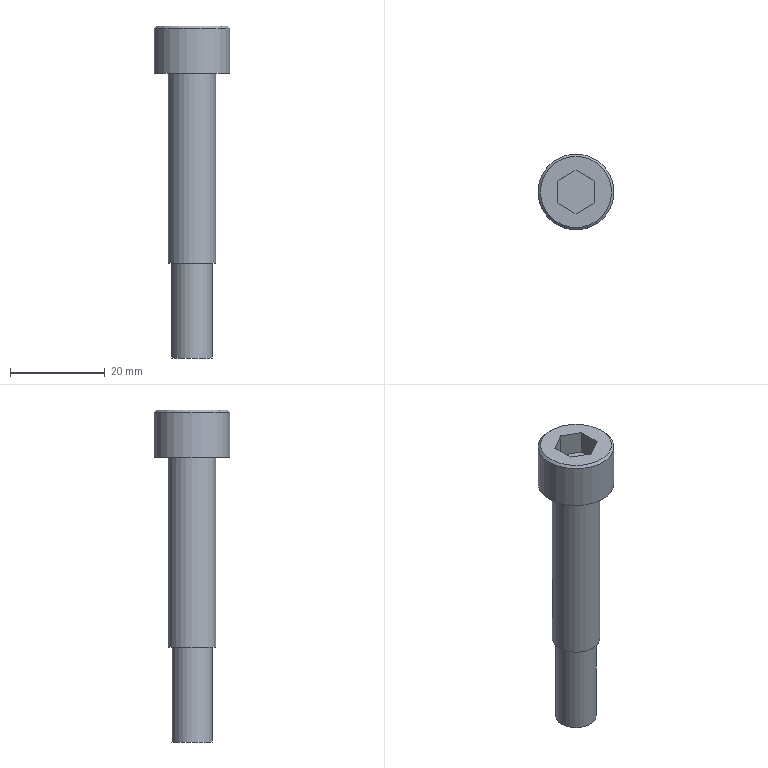Part | STEP file | M6-40_id1114_x_t | 1 solid | 15 faces | box 16 x 16 x 70 mm | volume 6004 mm3 | plane 11 | cylinder 3 | cone 1 | commonest cylinder face diameters 8.5 x1 10 x1 16 x1
STEP:
#1=CARTESIAN_POINT('',(-349.25,-157.5,-47.));
#2=VERTEX_POINT('',#1);
#3=CARTESIAN_POINT('',(-345.,-157.5,-47.));
#4=DIRECTION('',(0.,0.,-1.));
#5=DIRECTION('',(-1.,0.,0.));
#6=AXIS2_PLACEMENT_3D('',#3,#4,#5);
#7=CIRCLE('',#6,4.25);
#8=EDGE_CURVE('',#2,#2,#7,.T.);
#9=ORIENTED_EDGE('',*,*,#8,.F.);
#10=EDGE_LOOP('',(#9));
#11=FACE_BOUND('',#10,.T.);
#12=CARTESIAN_POINT('',(-340.,-157.5,-47.));
#13=VERTEX_POINT('',#12);
#14=CARTESIAN_POINT('',(-345.,-157.5,-47.));
#15=DIRECTION('',(0.,0.,1.));
#16=DIRECTION('',(1.,0.,0.));
#17=AXIS2_PLACEMENT_3D('',#14,#15,#16);
#18=CIRCLE('',#17,5.);
#19=EDGE_CURVE('',#13,#13,#18,.T.);
#20=ORIENTED_EDGE('',*,*,#19,.F.);
#21=EDGE_LOOP('',(#20));
#22=FACE_BOUND('',#21,.T.);
#23=CARTESIAN_POINT('',(-345.,-157.5,-47.));
#24=DIRECTION('',(0.,0.,-1.));
#25=DIRECTION('',(-1.,0.,0.));
#26=AXIS2_PLACEMENT_3D('',#23,#24,#25);
#27=PLANE('',#26);
#28=ADVANCED_FACE('',(#11,#22),#27,.T.);
#29=CARTESIAN_POINT('',(-350.,-157.5,-7.));
#30=VERTEX_POINT('',#29);
#31=CARTESIAN_POINT('',(-345.,-157.5,-7.));
#32=DIRECTION('',(0.,0.,1.));
#33=DIRECTION('',(-1.,0.,0.));
#34=AXIS2_PLACEMENT_3D('',#31,#32,#33);
#35=CIRCLE('',#34,5.);
#36=EDGE_CURVE('',#30,#30,#35,.T.);
#37=ORIENTED_EDGE('',*,*,#36,.F.);
#38=EDGE_LOOP('',(#37));
#39=FACE_BOUND('',#38,.T.);
#40=ORIENTED_EDGE('',*,*,#19,.T.);
#41=EDGE_LOOP('',(#40));
#42=FACE_BOUND('',#41,.T.);
#43=CARTESIAN_POINT('',(-345.,-157.5,-47.));
#44=DIRECTION('',(0.,0.,1.));
#45=DIRECTION('',(1.,0.,0.));
#46=AXIS2_PLACEMENT_3D('',#43,#44,#45);
#47=CYLINDRICAL_SURFACE('',#46,5.);
#48=ADVANCED_FACE('',(#39,#42),#47,.T.);
#49=CARTESIAN_POINT('',(-337.5,-157.5,3.));
#50=VERTEX_POINT('',#49);
#51=CARTESIAN_POINT('',(-345.,-157.5,3.));
#52=DIRECTION('',(0.,0.,1.));
#53=DIRECTION('',(1.,0.,0.));
#54=AXIS2_PLACEMENT_3D('',#51,#52,#53);
#55=CIRCLE('',#54,7.5);
#56=EDGE_CURVE('',#50,#50,#55,.T.);
#57=ORIENTED_EDGE('',*,*,#56,.T.);
#58=EDGE_LOOP('',(#57));
#59=FACE_BOUND('',#58,.T.);
#60=CARTESIAN_POINT('',(-349.,-155.191,3.));
#61=VERTEX_POINT('',#60);
#62=CARTESIAN_POINT('',(-349.,-159.809,3.));
#63=VERTEX_POINT('',#62);
#64=CARTESIAN_POINT('',(-349.,-155.191,3.));
#65=DIRECTION('',(0.,-1.,0.));
#66=VECTOR('',#65,1.);
#67=LINE('',#64,#66);
#68=EDGE_CURVE('',#61,#63,#67,.T.);
#69=ORIENTED_EDGE('',*,*,#68,.F.);
#70=CARTESIAN_POINT('',(-345.,-152.881,3.));
#71=VERTEX_POINT('',#70);
#72=CARTESIAN_POINT('',(-345.,-152.881,3.));
#73=DIRECTION('',(-0.866,-0.5,0.));
#74=VECTOR('',#73,1.);
#75=LINE('',#72,#74);
#76=EDGE_CURVE('',#71,#61,#75,.T.);
#77=ORIENTED_EDGE('',*,*,#76,.F.);
#78=CARTESIAN_POINT('',(-341.,-155.191,3.));
#79=VERTEX_POINT('',#78);
#80=CARTESIAN_POINT('',(-341.,-155.191,3.));
#81=DIRECTION('',(-0.866,0.5,0.));
#82=VECTOR('',#81,1.);
#83=LINE('',#80,#82);
#84=EDGE_CURVE('',#79,#71,#83,.T.);
#85=ORIENTED_EDGE('',*,*,#84,.F.);
#86=CARTESIAN_POINT('',(-341.,-159.809,3.));
#87=VERTEX_POINT('',#86);
#88=CARTESIAN_POINT('',(-341.,-159.809,3.));
#89=DIRECTION('',(0.,1.,0.));
#90=VECTOR('',#89,1.);
#91=LINE('',#88,#90);
#92=EDGE_CURVE('',#87,#79,#91,.T.);
#93=ORIENTED_EDGE('',*,*,#92,.F.);
#94=CARTESIAN_POINT('',(-345.,-162.119,3.));
#95=VERTEX_POINT('',#94);
#96=CARTESIAN_POINT('',(-345.,-162.119,3.));
#97=DIRECTION('',(0.866,0.5,0.));
#98=VECTOR('',#97,1.);
#99=LINE('',#96,#98);
#100=EDGE_CURVE('',#95,#87,#99,.T.);
#101=ORIENTED_EDGE('',*,*,#100,.F.);
#102=CARTESIAN_POINT('',(-349.,-159.809,3.));
#103=DIRECTION('',(0.866,-0.5,0.));
#104=VECTOR('',#103,1.);
#105=LINE('',#102,#104);
#106=EDGE_CURVE('',#63,#95,#105,.T.);
#107=ORIENTED_EDGE('',*,*,#106,.F.);
#108=EDGE_LOOP('',(#69,#77,#85,#93,#101,#107));
#109=FACE_BOUND('',#108,.T.);
#110=CARTESIAN_POINT('',(-345.,-157.5,3.));
#111=DIRECTION('',(0.,0.,1.));
#112=DIRECTION('',(1.,0.,0.));
#113=AXIS2_PLACEMENT_3D('',#110,#111,#112);
#114=PLANE('',#113);
#115=ADVANCED_FACE('',(#59,#109),#114,.T.);
#116=ORIENTED_EDGE('',*,*,#36,.T.);
#117=EDGE_LOOP('',(#116));
#118=FACE_BOUND('',#117,.T.);
#119=CARTESIAN_POINT('',(-337.,-157.5,-7.));
#120=VERTEX_POINT('',#119);
#121=CARTESIAN_POINT('',(-345.,-157.5,-7.));
#122=DIRECTION('',(0.,0.,1.));
#123=DIRECTION('',(1.,0.,0.));
#124=AXIS2_PLACEMENT_3D('',#121,#122,#123);
#125=CIRCLE('',#124,8.);
#126=EDGE_CURVE('',#120,#120,#125,.T.);
#127=ORIENTED_EDGE('',*,*,#126,.F.);
#128=EDGE_LOOP('',(#127));
#129=FACE_BOUND('',#128,.T.);
#130=CARTESIAN_POINT('',(-345.,-157.5,-7.));
#131=DIRECTION('',(0.,0.,-1.));
#132=DIRECTION('',(-1.,0.,0.));
#133=AXIS2_PLACEMENT_3D('',#130,#131,#132);
#134=PLANE('',#133);
#135=ADVANCED_FACE('',(#118,#129),#134,.T.);
#136=CARTESIAN_POINT('',(-337.,-157.5,2.5));
#137=VERTEX_POINT('',#136);
#138=CARTESIAN_POINT('',(-345.,-157.5,2.5));
#139=DIRECTION('',(0.,0.,-1.));
#140=DIRECTION('',(1.,0.,0.));
#141=AXIS2_PLACEMENT_3D('',#138,#139,#140);
#142=CIRCLE('',#141,8.);
#143=EDGE_CURVE('',#137,#137,#142,.T.);
#144=ORIENTED_EDGE('',*,*,#143,.T.);
#145=EDGE_LOOP('',(#144));
#146=FACE_BOUND('',#145,.T.);
#147=ORIENTED_EDGE('',*,*,#126,.T.);
#148=EDGE_LOOP('',(#147));
#149=FACE_BOUND('',#148,.T.);
#150=CARTESIAN_POINT('',(-345.,-157.5,-7.));
#151=DIRECTION('',(0.,0.,1.));
#152=DIRECTION('',(1.,0.,0.));
#153=AXIS2_PLACEMENT_3D('',#150,#151,#152);
#154=CYLINDRICAL_SURFACE('',#153,8.);
#155=ADVANCED_FACE('',(#146,#149),#154,.T.);
#156=CARTESIAN_POINT('',(-340.75,-157.5,-67.));
#157=VERTEX_POINT('',#156);
#158=CARTESIAN_POINT('',(-345.,-157.5,-67.));
#159=DIRECTION('',(0.,0.,1.));
#160=DIRECTION('',(1.,0.,0.));
#161=AXIS2_PLACEMENT_3D('',#158,#159,#160);
#162=CIRCLE('',#161,4.25);
#163=EDGE_CURVE('',#157,#157,#162,.T.);
#164=ORIENTED_EDGE('',*,*,#163,.F.);
#165=EDGE_LOOP('',(#164));
#166=FACE_OUTER_BOUND('',#165,.T.);
#167=CARTESIAN_POINT('',(-345.,-157.5,-67.));
#168=DIRECTION('',(0.,0.,-1.));
#169=DIRECTION('',(-1.,0.,0.));
#170=AXIS2_PLACEMENT_3D('',#167,#168,#169);
#171=PLANE('',#170);
#172=ADVANCED_FACE('',(#166),#171,.T.);
#173=ORIENTED_EDGE('',*,*,#163,.T.);
#174=EDGE_LOOP('',(#173));
#175=FACE_BOUND('',#174,.T.);
#176=ORIENTED_EDGE('',*,*,#8,.T.);
#177=EDGE_LOOP('',(#176));
#178=FACE_BOUND('',#177,.T.);
#179=CARTESIAN_POINT('',(-345.,-157.5,-47.));
#180=DIRECTION('',(0.,0.,-1.));
#181=DIRECTION('',(1.,0.,0.));
#182=AXIS2_PLACEMENT_3D('',#179,#180,#181);
#183=CYLINDRICAL_SURFACE('',#182,4.25);
#184=ADVANCED_FACE('',(#175,#178),#183,.T.);
#185=ORIENTED_EDGE('',*,*,#68,.T.);
#186=CARTESIAN_POINT('',(-349.,-159.809,-2.));
#187=VERTEX_POINT('',#186);
#188=CARTESIAN_POINT('',(-349.,-159.809,-2.));
#189=DIRECTION('',(0.,0.,-1.));
#190=VECTOR('',#189,1.);
#191=LINE('',#188,#190);
#192=EDGE_CURVE('',#63,#187,#191,.T.);
#193=ORIENTED_EDGE('',*,*,#192,.T.);
#194=CARTESIAN_POINT('',(-349.,-155.191,-2.));
#195=VERTEX_POINT('',#194);
#196=CARTESIAN_POINT('',(-349.,-155.191,-2.));
#197=DIRECTION('',(0.,1.,0.));
#198=VECTOR('',#197,1.);
#199=LINE('',#196,#198);
#200=EDGE_CURVE('',#187,#195,#199,.T.);
#201=ORIENTED_EDGE('',*,*,#200,.T.);
#202=CARTESIAN_POINT('',(-349.,-155.191,-2.));
#203=DIRECTION('',(0.,0.,-1.));
#204=VECTOR('',#203,1.);
#205=LINE('',#202,#204);
#206=EDGE_CURVE('',#61,#195,#205,.T.);
#207=ORIENTED_EDGE('',*,*,#206,.F.);
#208=EDGE_LOOP('',(#185,#193,#201,#207));
#209=FACE_OUTER_BOUND('',#208,.T.);
#210=CARTESIAN_POINT('',(-349.,-155.191,-2.));
#211=DIRECTION('',(-1.,0.,0.));
#212=DIRECTION('',(0.,-1.,0.));
#213=AXIS2_PLACEMENT_3D('',#210,#211,#212);
#214=PLANE('',#213);
#215=ADVANCED_FACE('',(#209),#214,.F.);
#216=ORIENTED_EDGE('',*,*,#106,.T.);
#217=CARTESIAN_POINT('',(-345.,-162.119,-2.));
#218=VERTEX_POINT('',#217);
#219=CARTESIAN_POINT('',(-345.,-162.119,-2.));
#220=DIRECTION('',(0.,0.,-1.));
#221=VECTOR('',#220,1.);
#222=LINE('',#219,#221);
#223=EDGE_CURVE('',#95,#218,#222,.T.);
#224=ORIENTED_EDGE('',*,*,#223,.T.);
#225=CARTESIAN_POINT('',(-349.,-159.809,-2.));
#226=DIRECTION('',(-0.866,0.5,0.));
#227=VECTOR('',#226,1.);
#228=LINE('',#225,#227);
#229=EDGE_CURVE('',#218,#187,#228,.T.);
#230=ORIENTED_EDGE('',*,*,#229,.T.);
#231=ORIENTED_EDGE('',*,*,#192,.F.);
#232=EDGE_LOOP('',(#216,#224,#230,#231));
#233=FACE_OUTER_BOUND('',#232,.T.);
#234=CARTESIAN_POINT('',(-349.,-159.809,-2.));
#235=DIRECTION('',(-0.5,-0.866,0.));
#236=DIRECTION('',(0.866,-0.5,0.));
#237=AXIS2_PLACEMENT_3D('',#234,#235,#236);
#238=PLANE('',#237);
#239=ADVANCED_FACE('',(#233),#238,.F.);
#240=ORIENTED_EDGE('',*,*,#100,.T.);
#241=CARTESIAN_POINT('',(-341.,-159.809,-2.));
#242=VERTEX_POINT('',#241);
#243=CARTESIAN_POINT('',(-341.,-159.809,-2.));
#244=DIRECTION('',(0.,0.,-1.));
#245=VECTOR('',#244,1.);
#246=LINE('',#243,#245);
#247=EDGE_CURVE('',#87,#242,#246,.T.);
#248=ORIENTED_EDGE('',*,*,#247,.T.);
#249=CARTESIAN_POINT('',(-345.,-162.119,-2.));
#250=DIRECTION('',(-0.866,-0.5,0.));
#251=VECTOR('',#250,1.);
#252=LINE('',#249,#251);
#253=EDGE_CURVE('',#242,#218,#252,.T.);
#254=ORIENTED_EDGE('',*,*,#253,.T.);
#255=ORIENTED_EDGE('',*,*,#223,.F.);
#256=EDGE_LOOP('',(#240,#248,#254,#255));
#257=FACE_OUTER_BOUND('',#256,.T.);
#258=CARTESIAN_POINT('',(-345.,-162.119,-2.));
#259=DIRECTION('',(0.5,-0.866,0.));
#260=DIRECTION('',(0.866,0.5,0.));
#261=AXIS2_PLACEMENT_3D('',#258,#259,#260);
#262=PLANE('',#261);
#263=ADVANCED_FACE('',(#257),#262,.F.);
#264=ORIENTED_EDGE('',*,*,#92,.T.);
#265=CARTESIAN_POINT('',(-341.,-155.191,-2.));
#266=VERTEX_POINT('',#265);
#267=CARTESIAN_POINT('',(-341.,-155.191,-2.));
#268=DIRECTION('',(0.,0.,-1.));
#269=VECTOR('',#268,1.);
#270=LINE('',#267,#269);
#271=EDGE_CURVE('',#79,#266,#270,.T.);
#272=ORIENTED_EDGE('',*,*,#271,.T.);
#273=CARTESIAN_POINT('',(-341.,-159.809,-2.));
#274=DIRECTION('',(0.,-1.,0.));
#275=VECTOR('',#274,1.);
#276=LINE('',#273,#275);
#277=EDGE_CURVE('',#266,#242,#276,.T.);
#278=ORIENTED_EDGE('',*,*,#277,.T.);
#279=ORIENTED_EDGE('',*,*,#247,.F.);
#280=EDGE_LOOP('',(#264,#272,#278,#279));
#281=FACE_OUTER_BOUND('',#280,.T.);
#282=CARTESIAN_POINT('',(-341.,-159.809,-2.));
#283=DIRECTION('',(1.,0.,0.));
#284=DIRECTION('',(0.,1.,0.));
#285=AXIS2_PLACEMENT_3D('',#282,#283,#284);
#286=PLANE('',#285);
#287=ADVANCED_FACE('',(#281),#286,.F.);
#288=ORIENTED_EDGE('',*,*,#84,.T.);
#289=CARTESIAN_POINT('',(-345.,-152.881,-2.));
#290=VERTEX_POINT('',#289);
#291=CARTESIAN_POINT('',(-345.,-152.881,-2.));
#292=DIRECTION('',(0.,0.,-1.));
#293=VECTOR('',#292,1.);
#294=LINE('',#291,#293);
#295=EDGE_CURVE('',#71,#290,#294,.T.);
#296=ORIENTED_EDGE('',*,*,#295,.T.);
#297=CARTESIAN_POINT('',(-341.,-155.191,-2.));
#298=DIRECTION('',(0.866,-0.5,0.));
#299=VECTOR('',#298,1.);
#300=LINE('',#297,#299);
#301=EDGE_CURVE('',#290,#266,#300,.T.);
#302=ORIENTED_EDGE('',*,*,#301,.T.);
#303=ORIENTED_EDGE('',*,*,#271,.F.);
#304=EDGE_LOOP('',(#288,#296,#302,#303));
#305=FACE_OUTER_BOUND('',#304,.T.);
#306=CARTESIAN_POINT('',(-341.,-155.191,-2.));
#307=DIRECTION('',(0.5,0.866,0.));
#308=DIRECTION('',(-0.866,0.5,0.));
#309=AXIS2_PLACEMENT_3D('',#306,#307,#308);
#310=PLANE('',#309);
#311=ADVANCED_FACE('',(#305),#310,.F.);
#312=ORIENTED_EDGE('',*,*,#76,.T.);
#313=ORIENTED_EDGE('',*,*,#206,.T.);
#314=CARTESIAN_POINT('',(-345.,-152.881,-2.));
#315=DIRECTION('',(0.866,0.5,0.));
#316=VECTOR('',#315,1.);
#317=LINE('',#314,#316);
#318=EDGE_CURVE('',#195,#290,#317,.T.);
#319=ORIENTED_EDGE('',*,*,#318,.T.);
#320=ORIENTED_EDGE('',*,*,#295,.F.);
#321=EDGE_LOOP('',(#312,#313,#319,#320));
#322=FACE_OUTER_BOUND('',#321,.T.);
#323=CARTESIAN_POINT('',(-345.,-152.881,-2.));
#324=DIRECTION('',(-0.5,0.866,0.));
#325=DIRECTION('',(-0.866,-0.5,0.));
#326=AXIS2_PLACEMENT_3D('',#323,#324,#325);
#327=PLANE('',#326);
#328=ADVANCED_FACE('',(#322),#327,.F.);
#329=ORIENTED_EDGE('',*,*,#200,.F.);
#330=ORIENTED_EDGE('',*,*,#229,.F.);
#331=ORIENTED_EDGE('',*,*,#253,.F.);
#332=ORIENTED_EDGE('',*,*,#277,.F.);
#333=ORIENTED_EDGE('',*,*,#301,.F.);
#334=ORIENTED_EDGE('',*,*,#318,.F.);
#335=EDGE_LOOP('',(#329,#330,#331,#332,#333,#334));
#336=FACE_OUTER_BOUND('',#335,.T.);
#337=CARTESIAN_POINT('',(-345.,-157.5,-2.));
#338=DIRECTION('',(0.,0.,1.));
#339=DIRECTION('',(1.,0.,0.));
#340=AXIS2_PLACEMENT_3D('',#337,#338,#339);
#341=PLANE('',#340);
#342=ADVANCED_FACE('',(#336),#341,.T.);
#343=ORIENTED_EDGE('',*,*,#56,.F.);
#344=EDGE_LOOP('',(#343));
#345=FACE_BOUND('',#344,.T.);
#346=ORIENTED_EDGE('',*,*,#143,.F.);
#347=EDGE_LOOP('',(#346));
#348=FACE_BOUND('',#347,.T.);
#349=CARTESIAN_POINT('',(-345.,-157.5,2.5));
#350=DIRECTION('',(0.,0.,-1.));
#351=DIRECTION('',(-1.,0.,0.));
#352=AXIS2_PLACEMENT_3D('',#349,#350,#351);
#353=CONICAL_SURFACE('',#352,8.,45.);
#354=ADVANCED_FACE('',(#345,#348),#353,.T.);
#355=CLOSED_SHELL('',(#28,#48,#115,#135,#155,#172,#184,#215,#239,#263,#287,#311,#328,#342,#354));
#356=MANIFOLD_SOLID_BREP('',#355);
#357=(LENGTH_UNIT()NAMED_UNIT(*)SI_UNIT(.MILLI.,.METRE.));
#358=UNCERTAINTY_MEASURE_WITH_UNIT(LENGTH_MEASURE(0.00002),#357,'','');
#359=(NAMED_UNIT(*)PLANE_ANGLE_UNIT()SI_UNIT($,.RADIAN.));
#360=PLANE_ANGLE_MEASURE_WITH_UNIT(PLANE_ANGLE_MEASURE(0.01745),#359);
#361=DIMENSIONAL_EXPONENTS(0.,0.,0.,0.,0.,0.,0.);
#362=(CONVERSION_BASED_UNIT('DEGREE',#360)NAMED_UNIT(#361)PLANE_ANGLE_UNIT());
#363=(NAMED_UNIT(*)SI_UNIT($,.STERADIAN.)SOLID_ANGLE_UNIT());
#364=(GEOMETRIC_REPRESENTATION_CONTEXT(3)GLOBAL_UNCERTAINTY_ASSIGNED_CONTEXT((#358))GLOBAL_UNIT_ASSIGNED_CONTEXT((#357,#362,#363))REPRESENTATION_CONTEXT('',''));
#365=ADVANCED_BREP_SHAPE_REPRESENTATION('',(#356),#364);